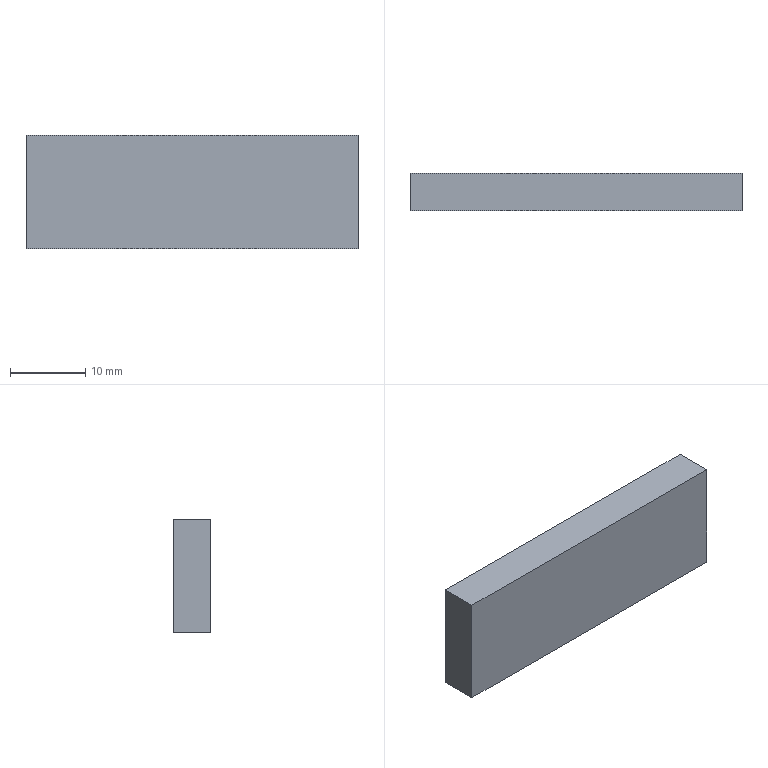Part | SolidWorks | features Extrusion 1 | 1 solid | 6 faces | box 44 x 5 x 15 mm | volume 3300 mm3 | plane 6
STEP:
#1=CARTESIAN_POINT('',(22.,0.,7.5));
#2=VERTEX_POINT('',#1);
#3=CARTESIAN_POINT('',(22.,0.,-7.5));
#4=VERTEX_POINT('',#3);
#5=CARTESIAN_POINT('',(22.,0.,7.5));
#6=DIRECTION('',(0.,0.,-1.));
#7=VECTOR('',#6,1000.);
#8=LINE('',#5,#7);
#9=EDGE_CURVE('',#2,#4,#8,.T.);
#10=ORIENTED_EDGE('',*,*,#9,.T.);
#11=CARTESIAN_POINT('',(22.,5.,-7.5));
#12=VERTEX_POINT('',#11);
#13=CARTESIAN_POINT('',(22.,5.,-7.5));
#14=DIRECTION('',(0.,-1.,0.));
#15=VECTOR('',#14,1000.);
#16=LINE('',#13,#15);
#17=EDGE_CURVE('',#12,#4,#16,.T.);
#18=ORIENTED_EDGE('',*,*,#17,.F.);
#19=CARTESIAN_POINT('',(22.,5.,7.5));
#20=VERTEX_POINT('',#19);
#21=CARTESIAN_POINT('',(22.,5.,7.5));
#22=DIRECTION('',(0.,0.,-1.));
#23=VECTOR('',#22,1000.);
#24=LINE('',#21,#23);
#25=EDGE_CURVE('',#20,#12,#24,.T.);
#26=ORIENTED_EDGE('',*,*,#25,.F.);
#27=CARTESIAN_POINT('',(22.,5.,7.5));
#28=DIRECTION('',(0.,-1.,0.));
#29=VECTOR('',#28,1000.);
#30=LINE('',#27,#29);
#31=EDGE_CURVE('',#20,#2,#30,.T.);
#32=ORIENTED_EDGE('',*,*,#31,.T.);
#33=EDGE_LOOP('',(#10,#18,#26,#32));
#34=FACE_OUTER_BOUND('',#33,.T.);
#35=CARTESIAN_POINT('',(22.,5.,7.5));
#36=DIRECTION('',(-1.,0.,0.));
#37=DIRECTION('',(0.,0.,1.));
#38=AXIS2_PLACEMENT_3D('',#35,#36,#37);
#39=PLANE('',#38);
#40=ADVANCED_FACE('',(#34),#39,.F.);
#41=CARTESIAN_POINT('',(-22.,0.,-7.5));
#42=VERTEX_POINT('',#41);
#43=CARTESIAN_POINT('',(-22.,0.,-7.5));
#44=DIRECTION('',(-1.,0.,0.));
#45=VECTOR('',#44,1000.);
#46=LINE('',#43,#45);
#47=EDGE_CURVE('',#4,#42,#46,.T.);
#48=ORIENTED_EDGE('',*,*,#47,.T.);
#49=CARTESIAN_POINT('',(-22.,5.,-7.5));
#50=VERTEX_POINT('',#49);
#51=CARTESIAN_POINT('',(-22.,5.,-7.5));
#52=DIRECTION('',(0.,-1.,0.));
#53=VECTOR('',#52,1000.);
#54=LINE('',#51,#53);
#55=EDGE_CURVE('',#50,#42,#54,.T.);
#56=ORIENTED_EDGE('',*,*,#55,.F.);
#57=CARTESIAN_POINT('',(-22.,5.,-7.5));
#58=DIRECTION('',(-1.,0.,0.));
#59=VECTOR('',#58,1000.);
#60=LINE('',#57,#59);
#61=EDGE_CURVE('',#12,#50,#60,.T.);
#62=ORIENTED_EDGE('',*,*,#61,.F.);
#63=ORIENTED_EDGE('',*,*,#17,.T.);
#64=EDGE_LOOP('',(#48,#56,#62,#63));
#65=FACE_OUTER_BOUND('',#64,.T.);
#66=CARTESIAN_POINT('',(-22.,5.,-7.5));
#67=DIRECTION('',(0.,0.,1.));
#68=DIRECTION('',(1.,0.,0.));
#69=AXIS2_PLACEMENT_3D('',#66,#67,#68);
#70=PLANE('',#69);
#71=ADVANCED_FACE('',(#65),#70,.F.);
#72=CARTESIAN_POINT('',(-22.,0.,7.5));
#73=VERTEX_POINT('',#72);
#74=CARTESIAN_POINT('',(-22.,0.,7.5));
#75=DIRECTION('',(0.,0.,1.));
#76=VECTOR('',#75,1000.);
#77=LINE('',#74,#76);
#78=EDGE_CURVE('',#42,#73,#77,.T.);
#79=ORIENTED_EDGE('',*,*,#78,.T.);
#80=CARTESIAN_POINT('',(-22.,5.,7.5));
#81=VERTEX_POINT('',#80);
#82=CARTESIAN_POINT('',(-22.,5.,7.5));
#83=DIRECTION('',(0.,-1.,0.));
#84=VECTOR('',#83,1000.);
#85=LINE('',#82,#84);
#86=EDGE_CURVE('',#81,#73,#85,.T.);
#87=ORIENTED_EDGE('',*,*,#86,.F.);
#88=CARTESIAN_POINT('',(-22.,5.,7.5));
#89=DIRECTION('',(0.,0.,1.));
#90=VECTOR('',#89,1000.);
#91=LINE('',#88,#90);
#92=EDGE_CURVE('',#50,#81,#91,.T.);
#93=ORIENTED_EDGE('',*,*,#92,.F.);
#94=ORIENTED_EDGE('',*,*,#55,.T.);
#95=EDGE_LOOP('',(#79,#87,#93,#94));
#96=FACE_OUTER_BOUND('',#95,.T.);
#97=CARTESIAN_POINT('',(-22.,5.,7.5));
#98=DIRECTION('',(1.,0.,0.));
#99=DIRECTION('',(0.,0.,-1.));
#100=AXIS2_PLACEMENT_3D('',#97,#98,#99);
#101=PLANE('',#100);
#102=ADVANCED_FACE('',(#96),#101,.F.);
#103=CARTESIAN_POINT('',(-22.,0.,7.5));
#104=DIRECTION('',(1.,0.,0.));
#105=VECTOR('',#104,1000.);
#106=LINE('',#103,#105);
#107=EDGE_CURVE('',#73,#2,#106,.T.);
#108=ORIENTED_EDGE('',*,*,#107,.T.);
#109=ORIENTED_EDGE('',*,*,#31,.F.);
#110=CARTESIAN_POINT('',(-22.,5.,7.5));
#111=DIRECTION('',(1.,0.,0.));
#112=VECTOR('',#111,1000.);
#113=LINE('',#110,#112);
#114=EDGE_CURVE('',#81,#20,#113,.T.);
#115=ORIENTED_EDGE('',*,*,#114,.F.);
#116=ORIENTED_EDGE('',*,*,#86,.T.);
#117=EDGE_LOOP('',(#108,#109,#115,#116));
#118=FACE_OUTER_BOUND('',#117,.T.);
#119=CARTESIAN_POINT('',(-22.,5.,7.5));
#120=DIRECTION('',(0.,0.,-1.));
#121=DIRECTION('',(-1.,0.,0.));
#122=AXIS2_PLACEMENT_3D('',#119,#120,#121);
#123=PLANE('',#122);
#124=ADVANCED_FACE('',(#118),#123,.F.);
#125=ORIENTED_EDGE('',*,*,#25,.T.);
#126=ORIENTED_EDGE('',*,*,#61,.T.);
#127=ORIENTED_EDGE('',*,*,#92,.T.);
#128=ORIENTED_EDGE('',*,*,#114,.T.);
#129=EDGE_LOOP('',(#125,#126,#127,#128));
#130=FACE_OUTER_BOUND('',#129,.T.);
#131=CARTESIAN_POINT('',(0.,5.,0.));
#132=DIRECTION('',(0.,-1.,0.));
#133=DIRECTION('',(0.,0.,-1.));
#134=AXIS2_PLACEMENT_3D('',#131,#132,#133);
#135=PLANE('',#134);
#136=ADVANCED_FACE('',(#130),#135,.F.);
#137=ORIENTED_EDGE('',*,*,#9,.F.);
#138=ORIENTED_EDGE('',*,*,#107,.F.);
#139=ORIENTED_EDGE('',*,*,#78,.F.);
#140=ORIENTED_EDGE('',*,*,#47,.F.);
#141=EDGE_LOOP('',(#137,#138,#139,#140));
#142=FACE_OUTER_BOUND('',#141,.T.);
#143=CARTESIAN_POINT('',(0.,0.,0.));
#144=DIRECTION('',(0.,-1.,0.));
#145=DIRECTION('',(0.,0.,-1.));
#146=AXIS2_PLACEMENT_3D('',#143,#144,#145);
#147=PLANE('',#146);
#148=ADVANCED_FACE('',(#142),#147,.T.);
#149=CLOSED_SHELL('',(#40,#71,#102,#124,#136,#148));
#150=MANIFOLD_SOLID_BREP('',#149);
#151=CARTESIAN_POINT('',(0.,0.,0.));
#152=DIRECTION('',(0.,0.,1.));
#153=DIRECTION('',(1.,0.,0.));
#154=AXIS2_PLACEMENT_3D('',#151,#152,#153);
#155=(LENGTH_UNIT()NAMED_UNIT(*)SI_UNIT(.MILLI.,.METRE.));
#156=UNCERTAINTY_MEASURE_WITH_UNIT(LENGTH_MEASURE(0.00001),#155,'','');
#157=(NAMED_UNIT(*)PLANE_ANGLE_UNIT()SI_UNIT($,.RADIAN.));
#158=(NAMED_UNIT(*)SI_UNIT($,.STERADIAN.)SOLID_ANGLE_UNIT());
#159=(GEOMETRIC_REPRESENTATION_CONTEXT(3)GLOBAL_UNCERTAINTY_ASSIGNED_CONTEXT((#156))GLOBAL_UNIT_ASSIGNED_CONTEXT((#155,#157,#158))REPRESENTATION_CONTEXT('',''));
#160=ADVANCED_BREP_SHAPE_REPRESENTATION('',(#150,#154),#159);